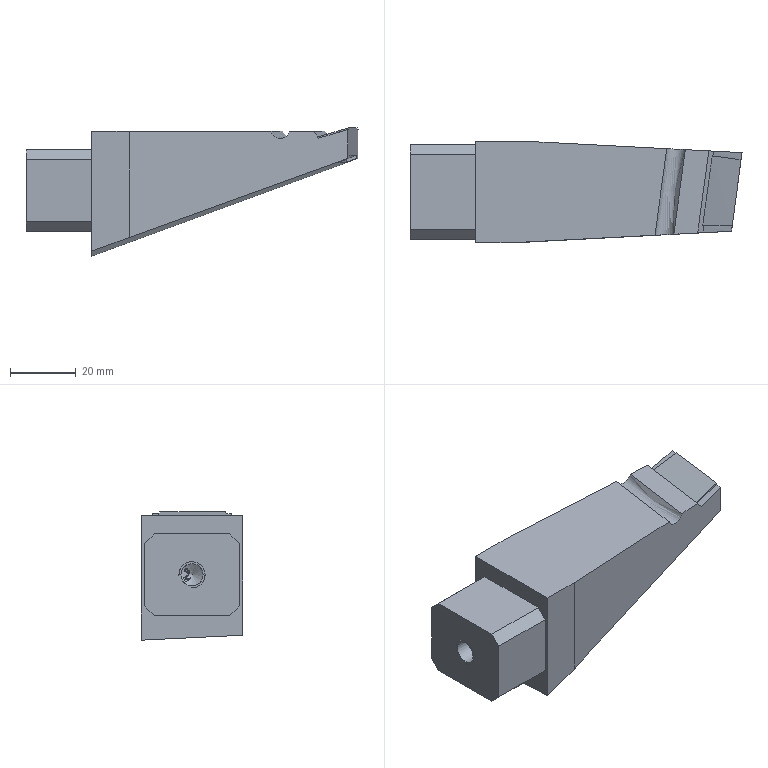Part | STEP file | P011002S003-002 | 1 solid | 64 faces | box 101.347 x 31 x 39.172 mm | volume 65480 mm3 | plane 36 | other 11 | spline 7 | cone 7 | cylinder 3 | commonest cylinder face diameters 6.8 x1 7.973 x1 8 x1